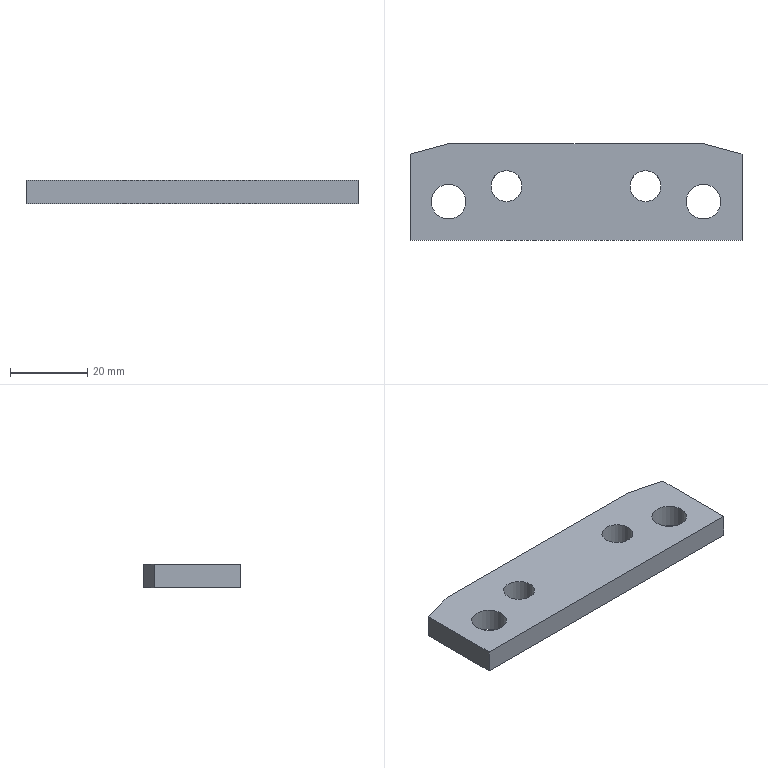Part | STEP file | gslz 2016.10.28-13_id722_x_t | 1 solid | 12 faces | box 86 x 25 x 6 mm | volume 11373 mm3 | plane 8 | cylinder 4 | commonest cylinder face diameters 8 x2 9 x2
STEP:
#1=CARTESIAN_POINT('',(0.,0.,0.));
#2=DIRECTION('',(0.,0.,1.));
#3=DIRECTION('',(1.,0.,0.));
#4=AXIS2_PLACEMENT_3D('',#1,#2,#3);
#5=CARTESIAN_POINT('',(1080.498,-278.75,6.));
#6=VERTEX_POINT('',#5);
#7=CARTESIAN_POINT('',(1088.498,-278.75,6.));
#8=VERTEX_POINT('',#7);
#9=CARTESIAN_POINT('',(1084.498,-278.75,6.));
#10=DIRECTION('',(0.,0.,-1.));
#11=DIRECTION('',(-1.,0.,0.));
#12=AXIS2_PLACEMENT_3D('',#9,#10,#11);
#13=CIRCLE('',#12,4.);
#14=CARTESIAN_POINT('',(1084.498,-278.75,-73.));
#15=DIRECTION('',(0.,0.,1.));
#16=DIRECTION('',(1.,0.,0.));
#17=AXIS2_PLACEMENT_3D('',#14,#15,#16);
#18=CYLINDRICAL_SURFACE('',#17,4.);
#19=CARTESIAN_POINT('',(3.142,79.));
#20=DIRECTION('',(-1.,0.));
#21=VECTOR('',#20,1.);
#22=LINE('',#19,#21);
#23=(GEOMETRIC_REPRESENTATION_CONTEXT(2)PARAMETRIC_REPRESENTATION_CONTEXT()REPRESENTATION_CONTEXT('',''));
#24=DEFINITIONAL_REPRESENTATION('',(#22),#23);
#25=PCURVE('',#18,#24);
#26=CARTESIAN_POINT('',(1032.498,-265.25,6.));
#27=DIRECTION('',(0.,0.,-1.));
#28=DIRECTION('',(-1.,0.,0.));
#29=AXIS2_PLACEMENT_3D('',#26,#27,#28);
#30=PLANE('',#29);
#31=CARTESIAN_POINT('',(-52.,-13.5));
#32=DIRECTION('',(1.,0.));
#33=AXIS2_PLACEMENT_2D('',#31,#32);
#34=CIRCLE('',#33,4.);
#35=(GEOMETRIC_REPRESENTATION_CONTEXT(2)PARAMETRIC_REPRESENTATION_CONTEXT()REPRESENTATION_CONTEXT('',''));
#36=DEFINITIONAL_REPRESENTATION('',(#34),#35);
#37=PCURVE('',#30,#36);
#38=SURFACE_CURVE('',#13,(#25,#37),.PCURVE_S1.);
#39=EDGE_CURVE('',#6,#8,#38,.T.);
#40=ORIENTED_EDGE('',*,*,#39,.T.);
#41=CARTESIAN_POINT('',(1088.498,-278.75,0.));
#42=VERTEX_POINT('',#41);
#43=CARTESIAN_POINT('',(1088.498,-278.75,0.));
#44=CARTESIAN_POINT('',(1088.498,-278.75,6.));
#45=B_SPLINE_CURVE_WITH_KNOTS('',1,(#43,#44),.UNSPECIFIED.,.F.,.F.,(2,2),(73.,79.),.PIECEWISE_BEZIER_KNOTS.);
#46=CARTESIAN_POINT('',(0.,0.));
#47=DIRECTION('',(0.,1.));
#48=VECTOR('',#47,1.);
#49=LINE('',#46,#48);
#50=(GEOMETRIC_REPRESENTATION_CONTEXT(2)PARAMETRIC_REPRESENTATION_CONTEXT()REPRESENTATION_CONTEXT('',''));
#51=DEFINITIONAL_REPRESENTATION('',(#49),#50);
#52=PCURVE('',#18,#51);
#53=CARTESIAN_POINT('',(6.283,0.));
#54=DIRECTION('',(0.,1.));
#55=VECTOR('',#54,1.);
#56=LINE('',#53,#55);
#57=(GEOMETRIC_REPRESENTATION_CONTEXT(2)PARAMETRIC_REPRESENTATION_CONTEXT()REPRESENTATION_CONTEXT('',''));
#58=DEFINITIONAL_REPRESENTATION('',(#56),#57);
#59=PCURVE('',#18,#58);
#60=SEAM_CURVE('',#45,(#52,#59),.PCURVE_S1.);
#61=EDGE_CURVE('',#42,#8,#60,.T.);
#62=ORIENTED_EDGE('',*,*,#61,.F.);
#63=CARTESIAN_POINT('',(1084.498,-278.75,0.));
#64=DIRECTION('',(0.,0.,1.));
#65=DIRECTION('',(1.,0.,0.));
#66=AXIS2_PLACEMENT_3D('',#63,#64,#65);
#67=CIRCLE('',#66,4.);
#68=CARTESIAN_POINT('',(0.,73.));
#69=DIRECTION('',(1.,0.));
#70=VECTOR('',#69,1.);
#71=LINE('',#68,#70);
#72=(GEOMETRIC_REPRESENTATION_CONTEXT(2)PARAMETRIC_REPRESENTATION_CONTEXT()REPRESENTATION_CONTEXT('',''));
#73=DEFINITIONAL_REPRESENTATION('',(#71),#72);
#74=PCURVE('',#18,#73);
#75=CARTESIAN_POINT('',(992.498,-295.75,0.));
#76=DIRECTION('',(0.,0.,1.));
#77=DIRECTION('',(1.,0.,0.));
#78=AXIS2_PLACEMENT_3D('',#75,#76,#77);
#79=PLANE('',#78);
#80=CARTESIAN_POINT('',(92.,17.));
#81=DIRECTION('',(1.,0.));
#82=AXIS2_PLACEMENT_2D('',#80,#81);
#83=CIRCLE('',#82,4.);
#84=(GEOMETRIC_REPRESENTATION_CONTEXT(2)PARAMETRIC_REPRESENTATION_CONTEXT()REPRESENTATION_CONTEXT('',''));
#85=DEFINITIONAL_REPRESENTATION('',(#83),#84);
#86=PCURVE('',#79,#85);
#87=SURFACE_CURVE('',#67,(#74,#86),.PCURVE_S1.);
#88=EDGE_CURVE('',#42,#42,#87,.T.);
#89=ORIENTED_EDGE('',*,*,#88,.T.);
#90=ORIENTED_EDGE('',*,*,#61,.T.);
#91=CARTESIAN_POINT('',(1084.498,-278.75,6.));
#92=DIRECTION('',(0.,0.,-1.));
#93=DIRECTION('',(-1.,0.,0.));
#94=AXIS2_PLACEMENT_3D('',#91,#92,#93);
#95=CIRCLE('',#94,4.);
#96=CARTESIAN_POINT('',(9.425,79.));
#97=DIRECTION('',(-1.,0.));
#98=VECTOR('',#97,1.);
#99=LINE('',#96,#98);
#100=(GEOMETRIC_REPRESENTATION_CONTEXT(2)PARAMETRIC_REPRESENTATION_CONTEXT()REPRESENTATION_CONTEXT('',''));
#101=DEFINITIONAL_REPRESENTATION('',(#99),#100);
#102=PCURVE('',#18,#101);
#103=CARTESIAN_POINT('',(-52.,-13.5));
#104=DIRECTION('',(1.,0.));
#105=AXIS2_PLACEMENT_2D('',#103,#104);
#106=CIRCLE('',#105,4.);
#107=(GEOMETRIC_REPRESENTATION_CONTEXT(2)PARAMETRIC_REPRESENTATION_CONTEXT()REPRESENTATION_CONTEXT('',''));
#108=DEFINITIONAL_REPRESENTATION('',(#106),#107);
#109=PCURVE('',#30,#108);
#110=SURFACE_CURVE('',#95,(#102,#109),.PCURVE_S1.);
#111=EDGE_CURVE('',#8,#6,#110,.T.);
#112=ORIENTED_EDGE('',*,*,#111,.T.);
#113=EDGE_LOOP('',(#40,#62,#89,#90,#112));
#114=FACE_BOUND('',#113,.F.);
#115=ADVANCED_FACE('',(#114),#18,.F.);
#116=CARTESIAN_POINT('',(1124.498,-278.75,6.));
#117=VERTEX_POINT('',#116);
#118=CARTESIAN_POINT('',(1116.498,-278.75,6.));
#119=VERTEX_POINT('',#118);
#120=CARTESIAN_POINT('',(1120.498,-278.75,6.));
#121=DIRECTION('',(0.,0.,1.));
#122=DIRECTION('',(-1.,0.,0.));
#123=AXIS2_PLACEMENT_3D('',#120,#121,#122);
#124=CIRCLE('',#123,4.);
#125=CARTESIAN_POINT('',(1120.498,-278.75,-73.));
#126=DIRECTION('',(0.,0.,1.));
#127=DIRECTION('',(1.,0.,0.));
#128=AXIS2_PLACEMENT_3D('',#125,#126,#127);
#129=CYLINDRICAL_SURFACE('',#128,4.);
#130=CARTESIAN_POINT('',(-3.142,79.));
#131=DIRECTION('',(1.,0.));
#132=VECTOR('',#131,1.);
#133=LINE('',#130,#132);
#134=(GEOMETRIC_REPRESENTATION_CONTEXT(2)PARAMETRIC_REPRESENTATION_CONTEXT()REPRESENTATION_CONTEXT('',''));
#135=DEFINITIONAL_REPRESENTATION('',(#133),#134);
#136=PCURVE('',#129,#135);
#137=CARTESIAN_POINT('',(-84.,-13.5));
#138=CARTESIAN_POINT('',(-84.,-20.428));
#139=CARTESIAN_POINT('',(-90.,-16.964));
#140=CARTESIAN_POINT('',(-96.,-13.5));
#141=CARTESIAN_POINT('',(-90.,-10.036));
#142=CARTESIAN_POINT('',(-84.,-6.572));
#143=CARTESIAN_POINT('',(-84.,-13.5));
#144=(BOUNDED_CURVE()B_SPLINE_CURVE(2,(#137,#138,#139,#140,#141,#142,#143),.UNSPECIFIED.,.T.,.F.)B_SPLINE_CURVE_WITH_KNOTS((1,2,2,2,2,1),(-2.094,0.,2.094,4.189,6.283,8.378),.UNSPECIFIED.)CURVE()GEOMETRIC_REPRESENTATION_ITEM()RATIONAL_B_SPLINE_CURVE((1.,0.5,1.,0.5,1.,0.5,1.))REPRESENTATION_ITEM(''));
#145=(GEOMETRIC_REPRESENTATION_CONTEXT(2)PARAMETRIC_REPRESENTATION_CONTEXT()REPRESENTATION_CONTEXT('',''));
#146=DEFINITIONAL_REPRESENTATION('',(#144),#145);
#147=PCURVE('',#30,#146);
#148=SURFACE_CURVE('',#124,(#136,#147),.PCURVE_S1.);
#149=EDGE_CURVE('',#117,#119,#148,.T.);
#150=ORIENTED_EDGE('',*,*,#149,.F.);
#151=CARTESIAN_POINT('',(1124.498,-278.75,0.));
#152=VERTEX_POINT('',#151);
#153=CARTESIAN_POINT('',(1124.498,-278.75,0.));
#154=CARTESIAN_POINT('',(1124.498,-278.75,6.));
#155=B_SPLINE_CURVE_WITH_KNOTS('',1,(#153,#154),.UNSPECIFIED.,.F.,.F.,(2,2),(73.,79.),.PIECEWISE_BEZIER_KNOTS.);
#156=CARTESIAN_POINT('',(0.,0.));
#157=DIRECTION('',(0.,1.));
#158=VECTOR('',#157,1.);
#159=LINE('',#156,#158);
#160=(GEOMETRIC_REPRESENTATION_CONTEXT(2)PARAMETRIC_REPRESENTATION_CONTEXT()REPRESENTATION_CONTEXT('',''));
#161=DEFINITIONAL_REPRESENTATION('',(#159),#160);
#162=PCURVE('',#129,#161);
#163=CARTESIAN_POINT('',(6.283,0.));
#164=DIRECTION('',(0.,1.));
#165=VECTOR('',#164,1.);
#166=LINE('',#163,#165);
#167=(GEOMETRIC_REPRESENTATION_CONTEXT(2)PARAMETRIC_REPRESENTATION_CONTEXT()REPRESENTATION_CONTEXT('',''));
#168=DEFINITIONAL_REPRESENTATION('',(#166),#167);
#169=PCURVE('',#129,#168);
#170=SEAM_CURVE('',#155,(#162,#169),.PCURVE_S1.);
#171=EDGE_CURVE('',#152,#117,#170,.T.);
#172=ORIENTED_EDGE('',*,*,#171,.F.);
#173=CARTESIAN_POINT('',(1120.498,-278.75,0.));
#174=DIRECTION('',(0.,0.,-1.));
#175=DIRECTION('',(1.,0.,0.));
#176=AXIS2_PLACEMENT_3D('',#173,#174,#175);
#177=CIRCLE('',#176,4.);
#178=CARTESIAN_POINT('',(6.283,73.));
#179=DIRECTION('',(-1.,0.));
#180=VECTOR('',#179,1.);
#181=LINE('',#178,#180);
#182=(GEOMETRIC_REPRESENTATION_CONTEXT(2)PARAMETRIC_REPRESENTATION_CONTEXT()REPRESENTATION_CONTEXT('',''));
#183=DEFINITIONAL_REPRESENTATION('',(#181),#182);
#184=PCURVE('',#129,#183);
#185=CARTESIAN_POINT('',(132.,17.));
#186=CARTESIAN_POINT('',(132.,10.072));
#187=CARTESIAN_POINT('',(126.,13.536));
#188=CARTESIAN_POINT('',(120.,17.));
#189=CARTESIAN_POINT('',(126.,20.464));
#190=CARTESIAN_POINT('',(132.,23.928));
#191=CARTESIAN_POINT('',(132.,17.));
#192=(BOUNDED_CURVE()B_SPLINE_CURVE(2,(#185,#186,#187,#188,#189,#190,#191),.UNSPECIFIED.,.T.,.F.)B_SPLINE_CURVE_WITH_KNOTS((1,2,2,2,2,1),(-2.094,0.,2.094,4.189,6.283,8.378),.UNSPECIFIED.)CURVE()GEOMETRIC_REPRESENTATION_ITEM()RATIONAL_B_SPLINE_CURVE((1.,0.5,1.,0.5,1.,0.5,1.))REPRESENTATION_ITEM(''));
#193=(GEOMETRIC_REPRESENTATION_CONTEXT(2)PARAMETRIC_REPRESENTATION_CONTEXT()REPRESENTATION_CONTEXT('',''));
#194=DEFINITIONAL_REPRESENTATION('',(#192),#193);
#195=PCURVE('',#79,#194);
#196=SURFACE_CURVE('',#177,(#184,#195),.PCURVE_S1.);
#197=EDGE_CURVE('',#152,#152,#196,.T.);
#198=ORIENTED_EDGE('',*,*,#197,.F.);
#199=ORIENTED_EDGE('',*,*,#171,.T.);
#200=CARTESIAN_POINT('',(1120.498,-278.75,6.));
#201=DIRECTION('',(0.,0.,1.));
#202=DIRECTION('',(-1.,0.,0.));
#203=AXIS2_PLACEMENT_3D('',#200,#201,#202);
#204=CIRCLE('',#203,4.);
#205=CARTESIAN_POINT('',(3.142,79.));
#206=DIRECTION('',(1.,0.));
#207=VECTOR('',#206,1.);
#208=LINE('',#205,#207);
#209=(GEOMETRIC_REPRESENTATION_CONTEXT(2)PARAMETRIC_REPRESENTATION_CONTEXT()REPRESENTATION_CONTEXT('',''));
#210=DEFINITIONAL_REPRESENTATION('',(#208),#209);
#211=PCURVE('',#129,#210);
#212=CARTESIAN_POINT('',(-84.,-13.5));
#213=CARTESIAN_POINT('',(-84.,-20.428));
#214=CARTESIAN_POINT('',(-90.,-16.964));
#215=CARTESIAN_POINT('',(-96.,-13.5));
#216=CARTESIAN_POINT('',(-90.,-10.036));
#217=CARTESIAN_POINT('',(-84.,-6.572));
#218=CARTESIAN_POINT('',(-84.,-13.5));
#219=(BOUNDED_CURVE()B_SPLINE_CURVE(2,(#212,#213,#214,#215,#216,#217,#218),.UNSPECIFIED.,.T.,.F.)B_SPLINE_CURVE_WITH_KNOTS((1,2,2,2,2,1),(-2.094,0.,2.094,4.189,6.283,8.378),.UNSPECIFIED.)CURVE()GEOMETRIC_REPRESENTATION_ITEM()RATIONAL_B_SPLINE_CURVE((1.,0.5,1.,0.5,1.,0.5,1.))REPRESENTATION_ITEM(''));
#220=(GEOMETRIC_REPRESENTATION_CONTEXT(2)PARAMETRIC_REPRESENTATION_CONTEXT()REPRESENTATION_CONTEXT('',''));
#221=DEFINITIONAL_REPRESENTATION('',(#219),#220);
#222=PCURVE('',#30,#221);
#223=SURFACE_CURVE('',#204,(#211,#222),.PCURVE_S1.);
#224=EDGE_CURVE('',#119,#117,#223,.T.);
#225=ORIENTED_EDGE('',*,*,#224,.F.);
#226=EDGE_LOOP('',(#150,#172,#198,#199,#225));
#227=FACE_BOUND('',#226,.F.);
#228=ADVANCED_FACE('',(#227),#129,.F.);
#229=CARTESIAN_POINT('',(1064.998,-282.75,6.));
#230=VERTEX_POINT('',#229);
#231=CARTESIAN_POINT('',(1069.498,-282.75,6.));
#232=DIRECTION('',(0.,0.,1.));
#233=DIRECTION('',(-1.,0.,0.));
#234=AXIS2_PLACEMENT_3D('',#231,#232,#233);
#235=CIRCLE('',#234,4.5);
#236=CARTESIAN_POINT('',(1069.498,-282.75,47.));
#237=DIRECTION('',(0.,0.,-1.));
#238=DIRECTION('',(-1.,0.,0.));
#239=AXIS2_PLACEMENT_3D('',#236,#237,#238);
#240=CYLINDRICAL_SURFACE('',#239,4.5);
#241=CARTESIAN_POINT('',(6.283,41.));
#242=DIRECTION('',(-1.,0.));
#243=VECTOR('',#242,1.);
#244=LINE('',#241,#243);
#245=(GEOMETRIC_REPRESENTATION_CONTEXT(2)PARAMETRIC_REPRESENTATION_CONTEXT()REPRESENTATION_CONTEXT('',''));
#246=DEFINITIONAL_REPRESENTATION('',(#244),#245);
#247=PCURVE('',#240,#246);
#248=CARTESIAN_POINT('',(-32.5,-17.5));
#249=CARTESIAN_POINT('',(-32.5,-25.294));
#250=CARTESIAN_POINT('',(-39.25,-21.397));
#251=CARTESIAN_POINT('',(-46.,-17.5));
#252=CARTESIAN_POINT('',(-39.25,-13.603));
#253=CARTESIAN_POINT('',(-32.5,-9.706));
#254=CARTESIAN_POINT('',(-32.5,-17.5));
#255=(BOUNDED_CURVE()B_SPLINE_CURVE(2,(#248,#249,#250,#251,#252,#253,#254),.UNSPECIFIED.,.T.,.F.)B_SPLINE_CURVE_WITH_KNOTS((1,2,2,2,2,1),(-2.094,0.,2.094,4.189,6.283,8.378),.UNSPECIFIED.)CURVE()GEOMETRIC_REPRESENTATION_ITEM()RATIONAL_B_SPLINE_CURVE((1.,0.5,1.,0.5,1.,0.5,1.))REPRESENTATION_ITEM(''));
#256=(GEOMETRIC_REPRESENTATION_CONTEXT(2)PARAMETRIC_REPRESENTATION_CONTEXT()REPRESENTATION_CONTEXT('',''));
#257=DEFINITIONAL_REPRESENTATION('',(#255),#256);
#258=PCURVE('',#30,#257);
#259=SURFACE_CURVE('',#235,(#247,#258),.PCURVE_S1.);
#260=EDGE_CURVE('',#230,#230,#259,.T.);
#261=ORIENTED_EDGE('',*,*,#260,.F.);
#262=CARTESIAN_POINT('',(1064.998,-282.75,0.));
#263=VERTEX_POINT('',#262);
#264=CARTESIAN_POINT('',(1064.998,-282.75,6.));
#265=CARTESIAN_POINT('',(1064.998,-282.75,0.));
#266=B_SPLINE_CURVE_WITH_KNOTS('',1,(#264,#265),.UNSPECIFIED.,.F.,.F.,(2,2),(41.,47.),.PIECEWISE_BEZIER_KNOTS.);
#267=CARTESIAN_POINT('',(6.283,0.));
#268=DIRECTION('',(0.,1.));
#269=VECTOR('',#268,1.);
#270=LINE('',#267,#269);
#271=(GEOMETRIC_REPRESENTATION_CONTEXT(2)PARAMETRIC_REPRESENTATION_CONTEXT()REPRESENTATION_CONTEXT('',''));
#272=DEFINITIONAL_REPRESENTATION('',(#270),#271);
#273=PCURVE('',#240,#272);
#274=CARTESIAN_POINT('',(0.,0.));
#275=DIRECTION('',(0.,1.));
#276=VECTOR('',#275,1.);
#277=LINE('',#274,#276);
#278=(GEOMETRIC_REPRESENTATION_CONTEXT(2)PARAMETRIC_REPRESENTATION_CONTEXT()REPRESENTATION_CONTEXT('',''));
#279=DEFINITIONAL_REPRESENTATION('',(#277),#278);
#280=PCURVE('',#240,#279);
#281=SEAM_CURVE('',#266,(#273,#280),.PCURVE_S1.);
#282=EDGE_CURVE('',#230,#263,#281,.T.);
#283=ORIENTED_EDGE('',*,*,#282,.T.);
#284=CARTESIAN_POINT('',(1073.998,-282.75,0.));
#285=VERTEX_POINT('',#284);
#286=CARTESIAN_POINT('',(1069.498,-282.75,0.));
#287=DIRECTION('',(0.,0.,-1.));
#288=DIRECTION('',(1.,0.,0.));
#289=AXIS2_PLACEMENT_3D('',#286,#287,#288);
#290=CIRCLE('',#289,4.5);
#291=CARTESIAN_POINT('',(3.142,47.));
#292=DIRECTION('',(1.,0.));
#293=VECTOR('',#292,1.);
#294=LINE('',#291,#293);
#295=(GEOMETRIC_REPRESENTATION_CONTEXT(2)PARAMETRIC_REPRESENTATION_CONTEXT()REPRESENTATION_CONTEXT('',''));
#296=DEFINITIONAL_REPRESENTATION('',(#294),#295);
#297=PCURVE('',#240,#296);
#298=CARTESIAN_POINT('',(81.5,13.));
#299=CARTESIAN_POINT('',(81.5,5.206));
#300=CARTESIAN_POINT('',(74.75,9.103));
#301=CARTESIAN_POINT('',(68.,13.));
#302=CARTESIAN_POINT('',(74.75,16.897));
#303=CARTESIAN_POINT('',(81.5,20.794));
#304=CARTESIAN_POINT('',(81.5,13.));
#305=(BOUNDED_CURVE()B_SPLINE_CURVE(2,(#298,#299,#300,#301,#302,#303,#304),.UNSPECIFIED.,.T.,.F.)B_SPLINE_CURVE_WITH_KNOTS((1,2,2,2,2,1),(-2.094,0.,2.094,4.189,6.283,8.378),.UNSPECIFIED.)CURVE()GEOMETRIC_REPRESENTATION_ITEM()RATIONAL_B_SPLINE_CURVE((1.,0.5,1.,0.5,1.,0.5,1.))REPRESENTATION_ITEM(''));
#306=(GEOMETRIC_REPRESENTATION_CONTEXT(2)PARAMETRIC_REPRESENTATION_CONTEXT()REPRESENTATION_CONTEXT('',''));
#307=DEFINITIONAL_REPRESENTATION('',(#305),#306);
#308=PCURVE('',#79,#307);
#309=SURFACE_CURVE('',#290,(#297,#308),.PCURVE_S1.);
#310=EDGE_CURVE('',#285,#263,#309,.T.);
#311=ORIENTED_EDGE('',*,*,#310,.F.);
#312=CARTESIAN_POINT('',(1069.498,-282.75,0.));
#313=DIRECTION('',(0.,0.,-1.));
#314=DIRECTION('',(1.,0.,0.));
#315=AXIS2_PLACEMENT_3D('',#312,#313,#314);
#316=CIRCLE('',#315,4.5);
#317=CARTESIAN_POINT('',(-3.142,47.));
#318=DIRECTION('',(1.,0.));
#319=VECTOR('',#318,1.);
#320=LINE('',#317,#319);
#321=(GEOMETRIC_REPRESENTATION_CONTEXT(2)PARAMETRIC_REPRESENTATION_CONTEXT()REPRESENTATION_CONTEXT('',''));
#322=DEFINITIONAL_REPRESENTATION('',(#320),#321);
#323=PCURVE('',#240,#322);
#324=CARTESIAN_POINT('',(81.5,13.));
#325=CARTESIAN_POINT('',(81.5,5.206));
#326=CARTESIAN_POINT('',(74.75,9.103));
#327=CARTESIAN_POINT('',(68.,13.));
#328=CARTESIAN_POINT('',(74.75,16.897));
#329=CARTESIAN_POINT('',(81.5,20.794));
#330=CARTESIAN_POINT('',(81.5,13.));
#331=(BOUNDED_CURVE()B_SPLINE_CURVE(2,(#324,#325,#326,#327,#328,#329,#330),.UNSPECIFIED.,.T.,.F.)B_SPLINE_CURVE_WITH_KNOTS((1,2,2,2,2,1),(-2.094,0.,2.094,4.189,6.283,8.378),.UNSPECIFIED.)CURVE()GEOMETRIC_REPRESENTATION_ITEM()RATIONAL_B_SPLINE_CURVE((1.,0.5,1.,0.5,1.,0.5,1.))REPRESENTATION_ITEM(''));
#332=(GEOMETRIC_REPRESENTATION_CONTEXT(2)PARAMETRIC_REPRESENTATION_CONTEXT()REPRESENTATION_CONTEXT('',''));
#333=DEFINITIONAL_REPRESENTATION('',(#331),#332);
#334=PCURVE('',#79,#333);
#335=SURFACE_CURVE('',#316,(#323,#334),.PCURVE_S1.);
#336=EDGE_CURVE('',#263,#285,#335,.T.);
#337=ORIENTED_EDGE('',*,*,#336,.F.);
#338=ORIENTED_EDGE('',*,*,#282,.F.);
#339=EDGE_LOOP('',(#261,#283,#311,#337,#338));
#340=FACE_BOUND('',#339,.F.);
#341=ADVANCED_FACE('',(#340),#240,.F.);
#342=CARTESIAN_POINT('',(1135.499,-267.75,0.));
#343=VERTEX_POINT('',#342);
#344=CARTESIAN_POINT('',(1135.499,-267.75,6.));
#345=VERTEX_POINT('',#344);
#346=CARTESIAN_POINT('',(1135.499,-267.75,8.));
#347=DIRECTION('',(0.,0.,1.));
#348=VECTOR('',#347,1.);
#349=LINE('',#346,#348);
#350=CARTESIAN_POINT('',(1002.5,-267.75,8.));
#351=DIRECTION('',(0.,-1.,0.));
#352=DIRECTION('',(0.,0.,1.));
#353=AXIS2_PLACEMENT_3D('',#350,#351,#352);
#354=PLANE('',#353);
#355=CARTESIAN_POINT('',(0.,-132.999));
#356=DIRECTION('',(1.,0.));
#357=VECTOR('',#356,1.);
#358=LINE('',#355,#357);
#359=(GEOMETRIC_REPRESENTATION_CONTEXT(2)PARAMETRIC_REPRESENTATION_CONTEXT()REPRESENTATION_CONTEXT('',''));
#360=DEFINITIONAL_REPRESENTATION('',(#358),#359);
#361=PCURVE('',#354,#360);
#362=CARTESIAN_POINT('',(1135.499,-267.75,8.));
#363=DIRECTION('',(-0.2588,-0.9659,0.));
#364=DIRECTION('',(-0.9659,0.2588,0.));
#365=AXIS2_PLACEMENT_3D('',#362,#363,#364);
#366=PLANE('',#365);
#367=CARTESIAN_POINT('',(0.,0.));
#368=DIRECTION('',(0.,-1.));
#369=VECTOR('',#368,1.);
#370=LINE('',#367,#369);
#371=(GEOMETRIC_REPRESENTATION_CONTEXT(2)PARAMETRIC_REPRESENTATION_CONTEXT()REPRESENTATION_CONTEXT('',''));
#372=DEFINITIONAL_REPRESENTATION('',(#370),#371);
#373=PCURVE('',#366,#372);
#374=SURFACE_CURVE('',#349,(#361,#373),.PCURVE_S1.);
#375=EDGE_CURVE('',#343,#345,#374,.T.);
#376=ORIENTED_EDGE('',*,*,#375,.F.);
#377=CARTESIAN_POINT('',(1069.5,-267.75,0.));
#378=VERTEX_POINT('',#377);
#379=CARTESIAN_POINT('',(1002.5,-267.75,0.));
#380=DIRECTION('',(1.,0.,0.));
#381=VECTOR('',#380,1.);
#382=LINE('',#379,#381);
#383=CARTESIAN_POINT('',(-8.,0.));
#384=DIRECTION('',(0.,-1.));
#385=VECTOR('',#384,1.);
#386=LINE('',#383,#385);
#387=(GEOMETRIC_REPRESENTATION_CONTEXT(2)PARAMETRIC_REPRESENTATION_CONTEXT()REPRESENTATION_CONTEXT('',''));
#388=DEFINITIONAL_REPRESENTATION('',(#386),#387);
#389=PCURVE('',#354,#388);
#390=CARTESIAN_POINT('',(10.002,28.));
#391=DIRECTION('',(1.,0.));
#392=VECTOR('',#391,1.);
#393=LINE('',#390,#392);
#394=(GEOMETRIC_REPRESENTATION_CONTEXT(2)PARAMETRIC_REPRESENTATION_CONTEXT()REPRESENTATION_CONTEXT('',''));
#395=DEFINITIONAL_REPRESENTATION('',(#393),#394);
#396=PCURVE('',#79,#395);
#397=SURFACE_CURVE('',#382,(#389,#396),.PCURVE_S1.);
#398=EDGE_CURVE('',#378,#343,#397,.T.);
#399=ORIENTED_EDGE('',*,*,#398,.F.);
#400=CARTESIAN_POINT('',(1069.5,-267.75,6.));
#401=VERTEX_POINT('',#400);
#402=CARTESIAN_POINT('',(1069.5,-267.75,8.));
#403=DIRECTION('',(0.,0.,1.));
#404=VECTOR('',#403,1.);
#405=LINE('',#402,#404);
#406=CARTESIAN_POINT('',(0.,-67.));
#407=DIRECTION('',(1.,0.));
#408=VECTOR('',#407,1.);
#409=LINE('',#406,#408);
#410=(GEOMETRIC_REPRESENTATION_CONTEXT(2)PARAMETRIC_REPRESENTATION_CONTEXT()REPRESENTATION_CONTEXT('',''));
#411=DEFINITIONAL_REPRESENTATION('',(#409),#410);
#412=PCURVE('',#354,#411);
#413=CARTESIAN_POINT('',(1059.498,-270.43,8.));
#414=DIRECTION('',(0.2588,-0.9659,0.));
#415=DIRECTION('',(-0.9659,-0.2588,0.));
#416=AXIS2_PLACEMENT_3D('',#413,#414,#415);
#417=PLANE('',#416);
#418=CARTESIAN_POINT('',(-10.355,0.));
#419=DIRECTION('',(0.,-1.));
#420=VECTOR('',#419,1.);
#421=LINE('',#418,#420);
#422=(GEOMETRIC_REPRESENTATION_CONTEXT(2)PARAMETRIC_REPRESENTATION_CONTEXT()REPRESENTATION_CONTEXT('',''));
#423=DEFINITIONAL_REPRESENTATION('',(#421),#422);
#424=PCURVE('',#417,#423);
#425=SURFACE_CURVE('',#405,(#412,#424),.PCURVE_S1.);
#426=EDGE_CURVE('',#378,#401,#425,.T.);
#427=ORIENTED_EDGE('',*,*,#426,.T.);
#428=CARTESIAN_POINT('',(1002.5,-267.75,6.));
#429=DIRECTION('',(-1.,0.,0.));
#430=VECTOR('',#429,1.);
#431=LINE('',#428,#430);
#432=CARTESIAN_POINT('',(-2.,0.));
#433=DIRECTION('',(0.,1.));
#434=VECTOR('',#433,1.);
#435=LINE('',#432,#434);
#436=(GEOMETRIC_REPRESENTATION_CONTEXT(2)PARAMETRIC_REPRESENTATION_CONTEXT()REPRESENTATION_CONTEXT('',''));
#437=DEFINITIONAL_REPRESENTATION('',(#435),#436);
#438=PCURVE('',#354,#437);
#439=CARTESIAN_POINT('',(29.998,-2.5));
#440=DIRECTION('',(1.,0.));
#441=VECTOR('',#440,1.);
#442=LINE('',#439,#441);
#443=(GEOMETRIC_REPRESENTATION_CONTEXT(2)PARAMETRIC_REPRESENTATION_CONTEXT()REPRESENTATION_CONTEXT('',''));
#444=DEFINITIONAL_REPRESENTATION('',(#442),#443);
#445=PCURVE('',#30,#444);
#446=SURFACE_CURVE('',#431,(#438,#445),.PCURVE_S1.);
#447=EDGE_CURVE('',#345,#401,#446,.T.);
#448=ORIENTED_EDGE('',*,*,#447,.F.);
#449=EDGE_LOOP('',(#376,#399,#427,#448));
#450=FACE_BOUND('',#449,.T.);
#451=ADVANCED_FACE('',(#450),#354,.F.);
#452=CARTESIAN_POINT('',(1145.498,-270.429,6.));
#453=VERTEX_POINT('',#452);
#454=CARTESIAN_POINT('',(1145.498,-270.429,0.));
#455=VERTEX_POINT('',#454);
#456=CARTESIAN_POINT('',(1145.498,-270.429,8.));
#457=DIRECTION('',(0.,0.,-1.));
#458=VECTOR('',#457,1.);
#459=LINE('',#456,#458);
#460=CARTESIAN_POINT('',(-10.352,0.));
#461=DIRECTION('',(0.,1.));
#462=VECTOR('',#461,1.);
#463=LINE('',#460,#462);
#464=(GEOMETRIC_REPRESENTATION_CONTEXT(2)PARAMETRIC_REPRESENTATION_CONTEXT()REPRESENTATION_CONTEXT('',''));
#465=DEFINITIONAL_REPRESENTATION('',(#463),#464);
#466=PCURVE('',#366,#465);
#467=CARTESIAN_POINT('',(1145.498,-262.75,16.));
#468=DIRECTION('',(-1.,0.,0.));
#469=DIRECTION('',(0.,0.,1.));
#470=AXIS2_PLACEMENT_3D('',#467,#468,#469);
#471=PLANE('',#470);
#472=CARTESIAN_POINT('',(-8.,-7.679));
#473=DIRECTION('',(-1.,0.));
#474=VECTOR('',#473,1.);
#475=LINE('',#472,#474);
#476=(GEOMETRIC_REPRESENTATION_CONTEXT(2)PARAMETRIC_REPRESENTATION_CONTEXT()REPRESENTATION_CONTEXT('',''));
#477=DEFINITIONAL_REPRESENTATION('',(#475),#476);
#478=PCURVE('',#471,#477);
#479=SURFACE_CURVE('',#459,(#466,#478),.PCURVE_S1.);
#480=EDGE_CURVE('',#453,#455,#479,.T.);
#481=ORIENTED_EDGE('',*,*,#480,.T.);
#482=CARTESIAN_POINT('',(1135.499,-267.75,0.));
#483=DIRECTION('',(0.9659,-0.2588,0.));
#484=VECTOR('',#483,1.);
#485=LINE('',#482,#484);
#486=CARTESIAN_POINT('',(0.,8.));
#487=DIRECTION('',(-1.,0.));
#488=VECTOR('',#487,1.);
#489=LINE('',#486,#488);
#490=(GEOMETRIC_REPRESENTATION_CONTEXT(2)PARAMETRIC_REPRESENTATION_CONTEXT()REPRESENTATION_CONTEXT('',''));
#491=DEFINITIONAL_REPRESENTATION('',(#489),#490);
#492=PCURVE('',#366,#491);
#493=CARTESIAN_POINT('',(143.001,28.));
#494=DIRECTION('',(0.9659,-0.2588));
#495=VECTOR('',#494,1.);
#496=LINE('',#493,#495);
#497=(GEOMETRIC_REPRESENTATION_CONTEXT(2)PARAMETRIC_REPRESENTATION_CONTEXT()REPRESENTATION_CONTEXT('',''));
#498=DEFINITIONAL_REPRESENTATION('',(#496),#497);
#499=PCURVE('',#79,#498);
#500=SURFACE_CURVE('',#485,(#492,#499),.PCURVE_S1.);
#501=EDGE_CURVE('',#343,#455,#500,.T.);
#502=ORIENTED_EDGE('',*,*,#501,.F.);
#503=ORIENTED_EDGE('',*,*,#375,.T.);
#504=CARTESIAN_POINT('',(1135.499,-267.75,6.));
#505=DIRECTION('',(-0.9659,0.2588,0.));
#506=VECTOR('',#505,1.);
#507=LINE('',#504,#506);
#508=CARTESIAN_POINT('',(0.,2.));
#509=DIRECTION('',(1.,0.));
#510=VECTOR('',#509,1.);
#511=LINE('',#508,#510);
#512=(GEOMETRIC_REPRESENTATION_CONTEXT(2)PARAMETRIC_REPRESENTATION_CONTEXT()REPRESENTATION_CONTEXT('',''));
#513=DEFINITIONAL_REPRESENTATION('',(#511),#512);
#514=PCURVE('',#366,#513);
#515=CARTESIAN_POINT('',(-103.001,-2.5));
#516=DIRECTION('',(0.9659,0.2588));
#517=VECTOR('',#516,1.);
#518=LINE('',#515,#517);
#519=(GEOMETRIC_REPRESENTATION_CONTEXT(2)PARAMETRIC_REPRESENTATION_CONTEXT()REPRESENTATION_CONTEXT('',''));
#520=DEFINITIONAL_REPRESENTATION('',(#518),#519);
#521=PCURVE('',#30,#520);
#522=SURFACE_CURVE('',#507,(#514,#521),.PCURVE_S1.);
#523=EDGE_CURVE('',#453,#345,#522,.T.);
#524=ORIENTED_EDGE('',*,*,#523,.F.);
#525=EDGE_LOOP('',(#481,#502,#503,#524));
#526=FACE_BOUND('',#525,.T.);
#527=ADVANCED_FACE('',(#526),#366,.F.);
#528=CARTESIAN_POINT('',(1145.498,-292.75,6.));
#529=VERTEX_POINT('',#528);
#530=CARTESIAN_POINT('',(1145.498,-292.75,0.));
#531=VERTEX_POINT('',#530);
#532=CARTESIAN_POINT('',(1145.498,-292.75,16.));
#533=DIRECTION('',(0.,0.,-1.));
#534=VECTOR('',#533,1.);
#535=LINE('',#532,#534);
#536=CARTESIAN_POINT('',(0.,-30.));
#537=DIRECTION('',(-1.,0.));
#538=VECTOR('',#537,1.);
#539=LINE('',#536,#538);
#540=(GEOMETRIC_REPRESENTATION_CONTEXT(2)PARAMETRIC_REPRESENTATION_CONTEXT()REPRESENTATION_CONTEXT('',''));
#541=DEFINITIONAL_REPRESENTATION('',(#539),#540);
#542=PCURVE('',#471,#541);
#543=CARTESIAN_POINT('',(1072.498,-292.75,16.));
#544=DIRECTION('',(0.,1.,0.));
#545=DIRECTION('',(0.,0.,-1.));
#546=AXIS2_PLACEMENT_3D('',#543,#544,#545);
#547=PLANE('',#546);
#548=CARTESIAN_POINT('',(0.,-73.));
#549=DIRECTION('',(1.,0.));
#550=VECTOR('',#549,1.);
#551=LINE('',#548,#550);
#552=(GEOMETRIC_REPRESENTATION_CONTEXT(2)PARAMETRIC_REPRESENTATION_CONTEXT()REPRESENTATION_CONTEXT('',''));
#553=DEFINITIONAL_REPRESENTATION('',(#551),#552);
#554=PCURVE('',#547,#553);
#555=SURFACE_CURVE('',#535,(#542,#554),.PCURVE_S1.);
#556=EDGE_CURVE('',#529,#531,#555,.T.);
#557=ORIENTED_EDGE('',*,*,#556,.T.);
#558=CARTESIAN_POINT('',(1145.498,-262.75,0.));
#559=DIRECTION('',(0.,-1.,0.));
#560=VECTOR('',#559,1.);
#561=LINE('',#558,#560);
#562=CARTESIAN_POINT('',(-16.,0.));
#563=DIRECTION('',(0.,-1.));
#564=VECTOR('',#563,1.);
#565=LINE('',#562,#564);
#566=(GEOMETRIC_REPRESENTATION_CONTEXT(2)PARAMETRIC_REPRESENTATION_CONTEXT()REPRESENTATION_CONTEXT('',''));
#567=DEFINITIONAL_REPRESENTATION('',(#565),#566);
#568=PCURVE('',#471,#567);
#569=CARTESIAN_POINT('',(153.,33.));
#570=DIRECTION('',(0.,-1.));
#571=VECTOR('',#570,1.);
#572=LINE('',#569,#571);
#573=(GEOMETRIC_REPRESENTATION_CONTEXT(2)PARAMETRIC_REPRESENTATION_CONTEXT()REPRESENTATION_CONTEXT('',''));
#574=DEFINITIONAL_REPRESENTATION('',(#572),#573);
#575=PCURVE('',#79,#574);
#576=SURFACE_CURVE('',#561,(#568,#575),.PCURVE_S1.);
#577=EDGE_CURVE('',#455,#531,#576,.T.);
#578=ORIENTED_EDGE('',*,*,#577,.F.);
#579=ORIENTED_EDGE('',*,*,#480,.F.);
#580=CARTESIAN_POINT('',(1145.498,-262.75,6.));
#581=DIRECTION('',(0.,1.,0.));
#582=VECTOR('',#581,1.);
#583=LINE('',#580,#582);
#584=CARTESIAN_POINT('',(-10.,0.));
#585=DIRECTION('',(0.,1.));
#586=VECTOR('',#585,1.);
#587=LINE('',#584,#586);
#588=(GEOMETRIC_REPRESENTATION_CONTEXT(2)PARAMETRIC_REPRESENTATION_CONTEXT()REPRESENTATION_CONTEXT('',''));
#589=DEFINITIONAL_REPRESENTATION('',(#587),#588);
#590=PCURVE('',#471,#589);
#591=CARTESIAN_POINT('',(-113.,2.5));
#592=DIRECTION('',(0.,1.));
#593=VECTOR('',#592,1.);
#594=LINE('',#591,#593);
#595=(GEOMETRIC_REPRESENTATION_CONTEXT(2)PARAMETRIC_REPRESENTATION_CONTEXT()REPRESENTATION_CONTEXT('',''));
#596=DEFINITIONAL_REPRESENTATION('',(#594),#595);
#597=PCURVE('',#30,#596);
#598=SURFACE_CURVE('',#583,(#590,#597),.PCURVE_S1.);
#599=EDGE_CURVE('',#529,#453,#598,.T.);
#600=ORIENTED_EDGE('',*,*,#599,.F.);
#601=EDGE_LOOP('',(#557,#578,#579,#600));
#602=FACE_BOUND('',#601,.T.);
#603=ADVANCED_FACE('',(#602),#471,.F.);
#604=CARTESIAN_POINT('',(1059.498,-292.75,6.));
#605=VERTEX_POINT('',#604);
#606=CARTESIAN_POINT('',(1059.498,-292.75,0.));
#607=VERTEX_POINT('',#606);
#608=CARTESIAN_POINT('',(1059.498,-292.75,16.));
#609=DIRECTION('',(0.,0.,-1.));
#610=VECTOR('',#609,1.);
#611=LINE('',#608,#610);
#612=CARTESIAN_POINT('',(0.,13.));
#613=DIRECTION('',(1.,0.));
#614=VECTOR('',#613,1.);
#615=LINE('',#612,#614);
#616=(GEOMETRIC_REPRESENTATION_CONTEXT(2)PARAMETRIC_REPRESENTATION_CONTEXT()REPRESENTATION_CONTEXT('',''));
#617=DEFINITIONAL_REPRESENTATION('',(#615),#616);
#618=PCURVE('',#547,#617);
#619=CARTESIAN_POINT('',(1059.498,-295.75,16.));
#620=DIRECTION('',(1.,0.,0.));
#621=DIRECTION('',(0.,0.,-1.));
#622=AXIS2_PLACEMENT_3D('',#619,#620,#621);
#623=PLANE('',#622);
#624=CARTESIAN_POINT('',(0.,3.));
#625=DIRECTION('',(1.,0.));
#626=VECTOR('',#625,1.);
#627=LINE('',#624,#626);
#628=(GEOMETRIC_REPRESENTATION_CONTEXT(2)PARAMETRIC_REPRESENTATION_CONTEXT()REPRESENTATION_CONTEXT('',''));
#629=DEFINITIONAL_REPRESENTATION('',(#627),#628);
#630=PCURVE('',#623,#629);
#631=SURFACE_CURVE('',#611,(#618,#630),.PCURVE_S1.);
#632=EDGE_CURVE('',#605,#607,#631,.T.);
#633=ORIENTED_EDGE('',*,*,#632,.T.);
#634=CARTESIAN_POINT('',(1072.498,-292.75,0.));
#635=DIRECTION('',(-1.,0.,0.));
#636=VECTOR('',#635,1.);
#637=LINE('',#634,#636);
#638=CARTESIAN_POINT('',(16.,0.));
#639=DIRECTION('',(0.,1.));
#640=VECTOR('',#639,1.);
#641=LINE('',#638,#640);
#642=(GEOMETRIC_REPRESENTATION_CONTEXT(2)PARAMETRIC_REPRESENTATION_CONTEXT()REPRESENTATION_CONTEXT('',''));
#643=DEFINITIONAL_REPRESENTATION('',(#641),#642);
#644=PCURVE('',#547,#643);
#645=CARTESIAN_POINT('',(80.,3.));
#646=DIRECTION('',(-1.,0.));
#647=VECTOR('',#646,1.);
#648=LINE('',#645,#647);
#649=(GEOMETRIC_REPRESENTATION_CONTEXT(2)PARAMETRIC_REPRESENTATION_CONTEXT()REPRESENTATION_CONTEXT('',''));
#650=DEFINITIONAL_REPRESENTATION('',(#648),#649);
#651=PCURVE('',#79,#650);
#652=SURFACE_CURVE('',#637,(#644,#651),.PCURVE_S1.);
#653=EDGE_CURVE('',#531,#607,#652,.T.);
#654=ORIENTED_EDGE('',*,*,#653,.F.);
#655=ORIENTED_EDGE('',*,*,#556,.F.);
#656=CARTESIAN_POINT('',(1072.498,-292.75,6.));
#657=DIRECTION('',(1.,0.,0.));
#658=VECTOR('',#657,1.);
#659=LINE('',#656,#658);
#660=CARTESIAN_POINT('',(10.,0.));
#661=DIRECTION('',(0.,-1.));
#662=VECTOR('',#661,1.);
#663=LINE('',#660,#662);
#664=(GEOMETRIC_REPRESENTATION_CONTEXT(2)PARAMETRIC_REPRESENTATION_CONTEXT()REPRESENTATION_CONTEXT('',''));
#665=DEFINITIONAL_REPRESENTATION('',(#663),#664);
#666=PCURVE('',#547,#665);
#667=CARTESIAN_POINT('',(-40.,-27.5));
#668=DIRECTION('',(-1.,0.));
#669=VECTOR('',#668,1.);
#670=LINE('',#667,#669);
#671=(GEOMETRIC_REPRESENTATION_CONTEXT(2)PARAMETRIC_REPRESENTATION_CONTEXT()REPRESENTATION_CONTEXT('',''));
#672=DEFINITIONAL_REPRESENTATION('',(#670),#671);
#673=PCURVE('',#30,#672);
#674=SURFACE_CURVE('',#659,(#666,#673),.PCURVE_S1.);
#675=EDGE_CURVE('',#605,#529,#674,.T.);
#676=ORIENTED_EDGE('',*,*,#675,.F.);
#677=EDGE_LOOP('',(#633,#654,#655,#676));
#678=FACE_BOUND('',#677,.T.);
#679=ADVANCED_FACE('',(#678),#547,.F.);
#680=CARTESIAN_POINT('',(1059.498,-270.43,6.));
#681=VERTEX_POINT('',#680);
#682=CARTESIAN_POINT('',(1059.498,-270.43,0.));
#683=VERTEX_POINT('',#682);
#684=CARTESIAN_POINT('',(1059.498,-270.43,8.));
#685=DIRECTION('',(0.,0.,-1.));
#686=VECTOR('',#685,1.);
#687=LINE('',#684,#686);
#688=CARTESIAN_POINT('',(8.,25.32));
#689=DIRECTION('',(1.,0.));
#690=VECTOR('',#689,1.);
#691=LINE('',#688,#690);
#692=(GEOMETRIC_REPRESENTATION_CONTEXT(2)PARAMETRIC_REPRESENTATION_CONTEXT()REPRESENTATION_CONTEXT('',''));
#693=DEFINITIONAL_REPRESENTATION('',(#691),#692);
#694=PCURVE('',#623,#693);
#695=CARTESIAN_POINT('',(0.,0.));
#696=DIRECTION('',(0.,1.));
#697=VECTOR('',#696,1.);
#698=LINE('',#695,#697);
#699=(GEOMETRIC_REPRESENTATION_CONTEXT(2)PARAMETRIC_REPRESENTATION_CONTEXT()REPRESENTATION_CONTEXT('',''));
#700=DEFINITIONAL_REPRESENTATION('',(#698),#699);
#701=PCURVE('',#417,#700);
#702=SURFACE_CURVE('',#687,(#694,#701),.PCURVE_S1.);
#703=EDGE_CURVE('',#681,#683,#702,.T.);
#704=ORIENTED_EDGE('',*,*,#703,.T.);
#705=CARTESIAN_POINT('',(1059.498,-295.75,0.));
#706=DIRECTION('',(0.,1.,0.));
#707=VECTOR('',#706,1.);
#708=LINE('',#705,#707);
#709=CARTESIAN_POINT('',(16.,0.));
#710=DIRECTION('',(0.,1.));
#711=VECTOR('',#710,1.);
#712=LINE('',#709,#711);
#713=(GEOMETRIC_REPRESENTATION_CONTEXT(2)PARAMETRIC_REPRESENTATION_CONTEXT()REPRESENTATION_CONTEXT('',''));
#714=DEFINITIONAL_REPRESENTATION('',(#712),#713);
#715=PCURVE('',#623,#714);
#716=CARTESIAN_POINT('',(67.,0.));
#717=DIRECTION('',(0.,1.));
#718=VECTOR('',#717,1.);
#719=LINE('',#716,#718);
#720=(GEOMETRIC_REPRESENTATION_CONTEXT(2)PARAMETRIC_REPRESENTATION_CONTEXT()REPRESENTATION_CONTEXT('',''));
#721=DEFINITIONAL_REPRESENTATION('',(#719),#720);
#722=PCURVE('',#79,#721);
#723=SURFACE_CURVE('',#708,(#715,#722),.PCURVE_S1.);
#724=EDGE_CURVE('',#607,#683,#723,.T.);
#725=ORIENTED_EDGE('',*,*,#724,.F.);
#726=ORIENTED_EDGE('',*,*,#632,.F.);
#727=CARTESIAN_POINT('',(1059.498,-295.75,6.));
#728=DIRECTION('',(0.,-1.,0.));
#729=VECTOR('',#728,1.);
#730=LINE('',#727,#729);
#731=CARTESIAN_POINT('',(10.,0.));
#732=DIRECTION('',(0.,-1.));
#733=VECTOR('',#732,1.);
#734=LINE('',#731,#733);
#735=(GEOMETRIC_REPRESENTATION_CONTEXT(2)PARAMETRIC_REPRESENTATION_CONTEXT()REPRESENTATION_CONTEXT('',''));
#736=DEFINITIONAL_REPRESENTATION('',(#734),#735);
#737=PCURVE('',#623,#736);
#738=CARTESIAN_POINT('',(-27.,-30.5));
#739=DIRECTION('',(0.,-1.));
#740=VECTOR('',#739,1.);
#741=LINE('',#738,#740);
#742=(GEOMETRIC_REPRESENTATION_CONTEXT(2)PARAMETRIC_REPRESENTATION_CONTEXT()REPRESENTATION_CONTEXT('',''));
#743=DEFINITIONAL_REPRESENTATION('',(#741),#742);
#744=PCURVE('',#30,#743);
#745=SURFACE_CURVE('',#730,(#737,#744),.PCURVE_S1.);
#746=EDGE_CURVE('',#681,#605,#745,.T.);
#747=ORIENTED_EDGE('',*,*,#746,.F.);
#748=EDGE_LOOP('',(#704,#725,#726,#747));
#749=FACE_BOUND('',#748,.T.);
#750=ADVANCED_FACE('',(#749),#623,.F.);
#751=ORIENTED_EDGE('',*,*,#426,.F.);
#752=CARTESIAN_POINT('',(1059.498,-270.43,0.));
#753=DIRECTION('',(0.9659,0.2588,0.));
#754=VECTOR('',#753,1.);
#755=LINE('',#752,#754);
#756=CARTESIAN_POINT('',(0.,8.));
#757=DIRECTION('',(-1.,0.));
#758=VECTOR('',#757,1.);
#759=LINE('',#756,#758);
#760=(GEOMETRIC_REPRESENTATION_CONTEXT(2)PARAMETRIC_REPRESENTATION_CONTEXT()REPRESENTATION_CONTEXT('',''));
#761=DEFINITIONAL_REPRESENTATION('',(#759),#760);
#762=PCURVE('',#417,#761);
#763=CARTESIAN_POINT('',(67.,25.32));
#764=DIRECTION('',(0.9659,0.2588));
#765=VECTOR('',#764,1.);
#766=LINE('',#763,#765);
#767=(GEOMETRIC_REPRESENTATION_CONTEXT(2)PARAMETRIC_REPRESENTATION_CONTEXT()REPRESENTATION_CONTEXT('',''));
#768=DEFINITIONAL_REPRESENTATION('',(#766),#767);
#769=PCURVE('',#79,#768);
#770=SURFACE_CURVE('',#755,(#762,#769),.PCURVE_S1.);
#771=EDGE_CURVE('',#683,#378,#770,.T.);
#772=ORIENTED_EDGE('',*,*,#771,.F.);
#773=ORIENTED_EDGE('',*,*,#703,.F.);
#774=CARTESIAN_POINT('',(1059.498,-270.43,6.));
#775=DIRECTION('',(-0.9659,-0.2588,0.));
#776=VECTOR('',#775,1.);
#777=LINE('',#774,#776);
#778=CARTESIAN_POINT('',(0.,2.));
#779=DIRECTION('',(1.,0.));
#780=VECTOR('',#779,1.);
#781=LINE('',#778,#780);
#782=(GEOMETRIC_REPRESENTATION_CONTEXT(2)PARAMETRIC_REPRESENTATION_CONTEXT()REPRESENTATION_CONTEXT('',''));
#783=DEFINITIONAL_REPRESENTATION('',(#781),#782);
#784=PCURVE('',#417,#783);
#785=CARTESIAN_POINT('',(-27.,-5.18));
#786=DIRECTION('',(0.9659,-0.2588));
#787=VECTOR('',#786,1.);
#788=LINE('',#785,#787);
#789=(GEOMETRIC_REPRESENTATION_CONTEXT(2)PARAMETRIC_REPRESENTATION_CONTEXT()REPRESENTATION_CONTEXT('',''));
#790=DEFINITIONAL_REPRESENTATION('',(#788),#789);
#791=PCURVE('',#30,#790);
#792=SURFACE_CURVE('',#777,(#784,#791),.PCURVE_S1.);
#793=EDGE_CURVE('',#401,#681,#792,.T.);
#794=ORIENTED_EDGE('',*,*,#793,.F.);
#795=EDGE_LOOP('',(#751,#772,#773,#794));
#796=FACE_BOUND('',#795,.T.);
#797=ADVANCED_FACE('',(#796),#417,.F.);
#798=ORIENTED_EDGE('',*,*,#771,.T.);
#799=ORIENTED_EDGE('',*,*,#398,.T.);
#800=ORIENTED_EDGE('',*,*,#501,.T.);
#801=ORIENTED_EDGE('',*,*,#577,.T.);
#802=ORIENTED_EDGE('',*,*,#653,.T.);
#803=ORIENTED_EDGE('',*,*,#724,.T.);
#804=EDGE_LOOP('',(#798,#799,#800,#801,#802,#803));
#805=FACE_BOUND('',#804,.T.);
#806=ORIENTED_EDGE('',*,*,#310,.F.);
#807=ORIENTED_EDGE('',*,*,#336,.F.);
#808=EDGE_LOOP('',(#806,#807));
#809=FACE_BOUND('',#808,.T.);
#810=ORIENTED_EDGE('',*,*,#197,.F.);
#811=EDGE_LOOP('',(#810));
#812=FACE_BOUND('',#811,.T.);
#813=ORIENTED_EDGE('',*,*,#88,.T.);
#814=EDGE_LOOP('',(#813));
#815=FACE_BOUND('',#814,.T.);
#816=CARTESIAN_POINT('',(1139.998,-282.75,0.));
#817=VERTEX_POINT('',#816);
#818=CARTESIAN_POINT('',(1130.998,-282.75,0.));
#819=VERTEX_POINT('',#818);
#820=CARTESIAN_POINT('',(1135.498,-282.75,0.));
#821=DIRECTION('',(0.,0.,1.));
#822=DIRECTION('',(1.,0.,0.));
#823=AXIS2_PLACEMENT_3D('',#820,#821,#822);
#824=CIRCLE('',#823,4.5);
#825=CARTESIAN_POINT('',(143.,13.));
#826=DIRECTION('',(1.,0.));
#827=AXIS2_PLACEMENT_2D('',#825,#826);
#828=CIRCLE('',#827,4.5);
#829=(GEOMETRIC_REPRESENTATION_CONTEXT(2)PARAMETRIC_REPRESENTATION_CONTEXT()REPRESENTATION_CONTEXT('',''));
#830=DEFINITIONAL_REPRESENTATION('',(#828),#829);
#831=PCURVE('',#79,#830);
#832=CARTESIAN_POINT('',(1135.498,-282.75,47.));
#833=DIRECTION('',(0.,0.,-1.));
#834=DIRECTION('',(-1.,0.,0.));
#835=AXIS2_PLACEMENT_3D('',#832,#833,#834);
#836=CYLINDRICAL_SURFACE('',#835,4.5);
#837=CARTESIAN_POINT('',(3.142,47.));
#838=DIRECTION('',(-1.,0.));
#839=VECTOR('',#838,1.);
#840=LINE('',#837,#839);
#841=(GEOMETRIC_REPRESENTATION_CONTEXT(2)PARAMETRIC_REPRESENTATION_CONTEXT()REPRESENTATION_CONTEXT('',''));
#842=DEFINITIONAL_REPRESENTATION('',(#840),#841);
#843=PCURVE('',#836,#842);
#844=SURFACE_CURVE('',#824,(#831,#843),.PCURVE_S1.);
#845=EDGE_CURVE('',#817,#819,#844,.T.);
#846=ORIENTED_EDGE('',*,*,#845,.T.);
#847=CARTESIAN_POINT('',(1135.498,-282.75,0.));
#848=DIRECTION('',(0.,0.,1.));
#849=DIRECTION('',(1.,0.,0.));
#850=AXIS2_PLACEMENT_3D('',#847,#848,#849);
#851=CIRCLE('',#850,4.5);
#852=CARTESIAN_POINT('',(143.,13.));
#853=DIRECTION('',(1.,0.));
#854=AXIS2_PLACEMENT_2D('',#852,#853);
#855=CIRCLE('',#854,4.5);
#856=(GEOMETRIC_REPRESENTATION_CONTEXT(2)PARAMETRIC_REPRESENTATION_CONTEXT()REPRESENTATION_CONTEXT('',''));
#857=DEFINITIONAL_REPRESENTATION('',(#855),#856);
#858=PCURVE('',#79,#857);
#859=CARTESIAN_POINT('',(9.425,47.));
#860=DIRECTION('',(-1.,0.));
#861=VECTOR('',#860,1.);
#862=LINE('',#859,#861);
#863=(GEOMETRIC_REPRESENTATION_CONTEXT(2)PARAMETRIC_REPRESENTATION_CONTEXT()REPRESENTATION_CONTEXT('',''));
#864=DEFINITIONAL_REPRESENTATION('',(#862),#863);
#865=PCURVE('',#836,#864);
#866=SURFACE_CURVE('',#851,(#858,#865),.PCURVE_S1.);
#867=EDGE_CURVE('',#819,#817,#866,.T.);
#868=ORIENTED_EDGE('',*,*,#867,.T.);
#869=EDGE_LOOP('',(#846,#868));
#870=FACE_BOUND('',#869,.T.);
#871=ADVANCED_FACE('',(#805,#809,#812,#815,#870),#79,.F.);
#872=ORIENTED_EDGE('',*,*,#523,.T.);
#873=ORIENTED_EDGE('',*,*,#447,.T.);
#874=ORIENTED_EDGE('',*,*,#793,.T.);
#875=ORIENTED_EDGE('',*,*,#746,.T.);
#876=ORIENTED_EDGE('',*,*,#675,.T.);
#877=ORIENTED_EDGE('',*,*,#599,.T.);
#878=EDGE_LOOP('',(#872,#873,#874,#875,#876,#877));
#879=FACE_BOUND('',#878,.T.);
#880=ORIENTED_EDGE('',*,*,#260,.F.);
#881=EDGE_LOOP('',(#880));
#882=FACE_BOUND('',#881,.T.);
#883=ORIENTED_EDGE('',*,*,#224,.F.);
#884=ORIENTED_EDGE('',*,*,#149,.F.);
#885=EDGE_LOOP('',(#883,#884));
#886=FACE_BOUND('',#885,.T.);
#887=ORIENTED_EDGE('',*,*,#39,.T.);
#888=ORIENTED_EDGE('',*,*,#111,.T.);
#889=EDGE_LOOP('',(#887,#888));
#890=FACE_BOUND('',#889,.T.);
#891=CARTESIAN_POINT('',(1130.998,-282.75,6.));
#892=VERTEX_POINT('',#891);
#893=CARTESIAN_POINT('',(1135.498,-282.75,6.));
#894=DIRECTION('',(0.,0.,-1.));
#895=DIRECTION('',(-1.,0.,0.));
#896=AXIS2_PLACEMENT_3D('',#893,#894,#895);
#897=CIRCLE('',#896,4.5);
#898=CARTESIAN_POINT('',(-103.,-17.5));
#899=DIRECTION('',(1.,0.));
#900=AXIS2_PLACEMENT_2D('',#898,#899);
#901=CIRCLE('',#900,4.5);
#902=(GEOMETRIC_REPRESENTATION_CONTEXT(2)PARAMETRIC_REPRESENTATION_CONTEXT()REPRESENTATION_CONTEXT('',''));
#903=DEFINITIONAL_REPRESENTATION('',(#901),#902);
#904=PCURVE('',#30,#903);
#905=CARTESIAN_POINT('',(0.,41.));
#906=DIRECTION('',(1.,0.));
#907=VECTOR('',#906,1.);
#908=LINE('',#905,#907);
#909=(GEOMETRIC_REPRESENTATION_CONTEXT(2)PARAMETRIC_REPRESENTATION_CONTEXT()REPRESENTATION_CONTEXT('',''));
#910=DEFINITIONAL_REPRESENTATION('',(#908),#909);
#911=PCURVE('',#836,#910);
#912=SURFACE_CURVE('',#897,(#904,#911),.PCURVE_S1.);
#913=EDGE_CURVE('',#892,#892,#912,.T.);
#914=ORIENTED_EDGE('',*,*,#913,.T.);
#915=EDGE_LOOP('',(#914));
#916=FACE_BOUND('',#915,.T.);
#917=ADVANCED_FACE('',(#879,#882,#886,#890,#916),#30,.F.);
#918=ORIENTED_EDGE('',*,*,#913,.T.);
#919=CARTESIAN_POINT('',(1130.998,-282.75,6.));
#920=CARTESIAN_POINT('',(1130.998,-282.75,0.));
#921=B_SPLINE_CURVE_WITH_KNOTS('',1,(#919,#920),.UNSPECIFIED.,.F.,.F.,(2,2),(41.,47.),.PIECEWISE_BEZIER_KNOTS.);
#922=CARTESIAN_POINT('',(6.283,0.));
#923=DIRECTION('',(0.,1.));
#924=VECTOR('',#923,1.);
#925=LINE('',#922,#924);
#926=(GEOMETRIC_REPRESENTATION_CONTEXT(2)PARAMETRIC_REPRESENTATION_CONTEXT()REPRESENTATION_CONTEXT('',''));
#927=DEFINITIONAL_REPRESENTATION('',(#925),#926);
#928=PCURVE('',#836,#927);
#929=CARTESIAN_POINT('',(0.,0.));
#930=DIRECTION('',(0.,1.));
#931=VECTOR('',#930,1.);
#932=LINE('',#929,#931);
#933=(GEOMETRIC_REPRESENTATION_CONTEXT(2)PARAMETRIC_REPRESENTATION_CONTEXT()REPRESENTATION_CONTEXT('',''));
#934=DEFINITIONAL_REPRESENTATION('',(#932),#933);
#935=PCURVE('',#836,#934);
#936=SEAM_CURVE('',#921,(#928,#935),.PCURVE_S1.);
#937=EDGE_CURVE('',#892,#819,#936,.T.);
#938=ORIENTED_EDGE('',*,*,#937,.T.);
#939=ORIENTED_EDGE('',*,*,#867,.T.);
#940=ORIENTED_EDGE('',*,*,#845,.T.);
#941=ORIENTED_EDGE('',*,*,#937,.F.);
#942=EDGE_LOOP('',(#918,#938,#939,#940,#941));
#943=FACE_BOUND('',#942,.F.);
#944=ADVANCED_FACE('',(#943),#836,.F.);
#945=CLOSED_SHELL('',(#115,#228,#341,#451,#527,#603,#679,#750,#797,#871,#917,#944));
#946=MANIFOLD_SOLID_BREP('',#945);
#947=(LENGTH_UNIT()NAMED_UNIT(*)SI_UNIT(.MILLI.,.METRE.));
#948=UNCERTAINTY_MEASURE_WITH_UNIT(LENGTH_MEASURE(0.000002),#947,'','');
#949=(NAMED_UNIT(*)PLANE_ANGLE_UNIT()SI_UNIT($,.RADIAN.));
#950=(NAMED_UNIT(*)SI_UNIT($,.STERADIAN.)SOLID_ANGLE_UNIT());
#951=(GEOMETRIC_REPRESENTATION_CONTEXT(3)GLOBAL_UNCERTAINTY_ASSIGNED_CONTEXT((#948))GLOBAL_UNIT_ASSIGNED_CONTEXT((#947,#949,#950))REPRESENTATION_CONTEXT('',''));
#952=ADVANCED_BREP_SHAPE_REPRESENTATION('',(#4,#946),#951);